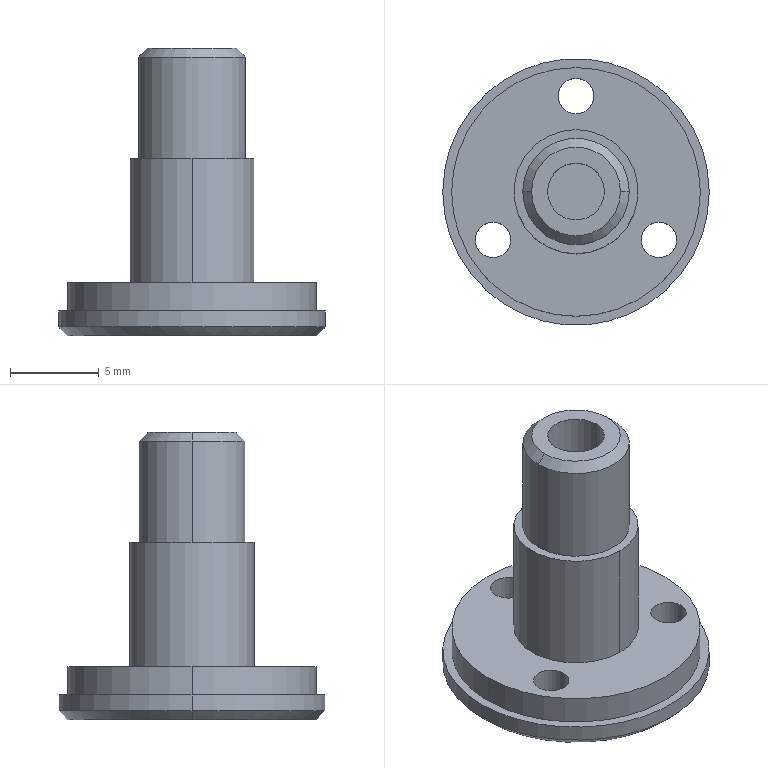Part | NX | features BREP 1 | 1 solid | 26 faces | box 15 x 15 x 16.2 mm | volume 821.71 mm3 | cylinder 16 | plane 6 | cone 4 | commonest cylinder face diameters 2 x6 3.2 x2 6 x2 7 x2 14 x2 15 x2
STEP:
#1=CARTESIAN_POINT('',(54.808,248.839,0.));
#2=VERTEX_POINT('',#1);
#3=CARTESIAN_POINT('',(49.808,248.839,0.));
#4=VERTEX_POINT('',#3);
#5=CARTESIAN_POINT('',(52.308,248.839,0.));
#6=DIRECTION('',(0.,0.,1.));
#7=DIRECTION('',(1.,0.,0.));
#8=AXIS2_PLACEMENT_3D('',#5,#6,#7);
#9=CIRCLE('',#8,2.5);
#10=EDGE_CURVE('',#2,#4,#9,.T.);
#11=ORIENTED_EDGE('',*,*,#10,.F.);
#12=CARTESIAN_POINT('',(55.308,248.839,-0.5));
#13=VERTEX_POINT('',#12);
#14=CARTESIAN_POINT('',(54.808,248.839,0.));
#15=DIRECTION('',(0.7071,0.,-0.7071));
#16=VECTOR('',#15,1000.);
#17=LINE('',#14,#16);
#18=EDGE_CURVE('',#13,#2,#17,.F.);
#19=ORIENTED_EDGE('',*,*,#18,.F.);
#20=CARTESIAN_POINT('',(49.308,248.839,-0.5));
#21=VERTEX_POINT('',#20);
#22=CARTESIAN_POINT('',(52.308,248.839,-0.5));
#23=DIRECTION('',(0.,0.,-1.));
#24=DIRECTION('',(1.,0.,0.));
#25=AXIS2_PLACEMENT_3D('',#22,#23,#24);
#26=CIRCLE('',#25,3.);
#27=EDGE_CURVE('',#21,#13,#26,.T.);
#28=ORIENTED_EDGE('',*,*,#27,.F.);
#29=CARTESIAN_POINT('',(49.808,248.839,0.));
#30=DIRECTION('',(-0.7071,0.,-0.7071));
#31=VECTOR('',#30,1000.);
#32=LINE('',#29,#31);
#33=EDGE_CURVE('',#21,#4,#32,.F.);
#34=ORIENTED_EDGE('',*,*,#33,.T.);
#35=EDGE_LOOP('',(#11,#19,#28,#34));
#36=FACE_BOUND('',#35,.T.);
#37=CARTESIAN_POINT('',(52.308,248.839,0.));
#38=DIRECTION('',(0.,0.,-1.));
#39=DIRECTION('',(1.,0.,0.));
#40=AXIS2_PLACEMENT_3D('',#37,#38,#39);
#41=CONICAL_SURFACE('',#40,2.5,0.7854);
#42=ADVANCED_FACE('',(#36),#41,.T.);
#43=CARTESIAN_POINT('',(50.708,248.839,-10.));
#44=VERTEX_POINT('',#43);
#45=CARTESIAN_POINT('',(53.908,248.839,-10.));
#46=VERTEX_POINT('',#45);
#47=CARTESIAN_POINT('',(52.308,248.839,-10.));
#48=DIRECTION('',(0.,0.,1.));
#49=DIRECTION('',(1.,0.,0.));
#50=AXIS2_PLACEMENT_3D('',#47,#48,#49);
#51=CIRCLE('',#50,1.6);
#52=EDGE_CURVE('',#44,#46,#51,.T.);
#53=ORIENTED_EDGE('',*,*,#52,.F.);
#54=CARTESIAN_POINT('',(50.708,248.839,0.));
#55=VERTEX_POINT('',#54);
#56=CARTESIAN_POINT('',(50.708,248.839,-10.));
#57=DIRECTION('',(0.,0.,1.));
#58=VECTOR('',#57,1000.);
#59=LINE('',#56,#58);
#60=EDGE_CURVE('',#44,#55,#59,.T.);
#61=ORIENTED_EDGE('',*,*,#60,.T.);
#62=CARTESIAN_POINT('',(53.908,248.839,0.));
#63=VERTEX_POINT('',#62);
#64=CARTESIAN_POINT('',(52.308,248.839,0.));
#65=DIRECTION('',(0.,0.,1.));
#66=DIRECTION('',(1.,0.,0.));
#67=AXIS2_PLACEMENT_3D('',#64,#65,#66);
#68=CIRCLE('',#67,1.6);
#69=EDGE_CURVE('',#55,#63,#68,.T.);
#70=ORIENTED_EDGE('',*,*,#69,.T.);
#71=CARTESIAN_POINT('',(53.908,248.839,-10.));
#72=DIRECTION('',(0.,0.,1.));
#73=VECTOR('',#72,1000.);
#74=LINE('',#71,#73);
#75=EDGE_CURVE('',#46,#63,#74,.T.);
#76=ORIENTED_EDGE('',*,*,#75,.F.);
#77=EDGE_LOOP('',(#53,#61,#70,#76));
#78=FACE_BOUND('',#77,.T.);
#79=CARTESIAN_POINT('',(52.308,248.839,-10.));
#80=DIRECTION('',(0.,0.,1.));
#81=DIRECTION('',(-1.,0.,0.));
#82=AXIS2_PLACEMENT_3D('',#79,#80,#81);
#83=CYLINDRICAL_SURFACE('',#82,1.6);
#84=ADVANCED_FACE('',(#78),#83,.F.);
#85=CARTESIAN_POINT('',(45.308,248.839,-16.2));
#86=VERTEX_POINT('',#85);
#87=CARTESIAN_POINT('',(59.308,248.839,-16.2));
#88=VERTEX_POINT('',#87);
#89=CARTESIAN_POINT('',(52.308,248.839,-16.2));
#90=DIRECTION('',(0.,0.,-1.));
#91=DIRECTION('',(0.,1.,0.));
#92=AXIS2_PLACEMENT_3D('',#89,#90,#91);
#93=CIRCLE('',#92,7.);
#94=EDGE_CURVE('',#86,#88,#93,.T.);
#95=ORIENTED_EDGE('',*,*,#94,.F.);
#96=CARTESIAN_POINT('',(44.808,248.839,-15.7));
#97=VERTEX_POINT('',#96);
#98=CARTESIAN_POINT('',(45.308,248.839,-16.2));
#99=DIRECTION('',(-0.7071,0.,0.7071));
#100=VECTOR('',#99,1000.);
#101=LINE('',#98,#100);
#102=EDGE_CURVE('',#86,#97,#101,.T.);
#103=ORIENTED_EDGE('',*,*,#102,.T.);
#104=CARTESIAN_POINT('',(59.808,248.839,-15.7));
#105=VERTEX_POINT('',#104);
#106=CARTESIAN_POINT('',(52.308,248.839,-15.7));
#107=DIRECTION('',(0.,0.,1.));
#108=DIRECTION('',(-1.,0.,0.));
#109=AXIS2_PLACEMENT_3D('',#106,#107,#108);
#110=CIRCLE('',#109,7.5);
#111=EDGE_CURVE('',#105,#97,#110,.T.);
#112=ORIENTED_EDGE('',*,*,#111,.F.);
#113=CARTESIAN_POINT('',(59.308,248.839,-16.2));
#114=DIRECTION('',(0.7071,0.,0.7071));
#115=VECTOR('',#114,1000.);
#116=LINE('',#113,#115);
#117=EDGE_CURVE('',#88,#105,#116,.T.);
#118=ORIENTED_EDGE('',*,*,#117,.F.);
#119=EDGE_LOOP('',(#95,#103,#112,#118));
#120=FACE_BOUND('',#119,.T.);
#121=CARTESIAN_POINT('',(52.308,248.839,-16.2));
#122=DIRECTION('',(0.,0.,1.));
#123=DIRECTION('',(-1.,0.,0.));
#124=AXIS2_PLACEMENT_3D('',#121,#122,#123);
#125=CONICAL_SURFACE('',#124,7.,0.7854);
#126=ADVANCED_FACE('',(#120),#125,.T.);
#127=ORIENTED_EDGE('',*,*,#111,.T.);
#128=CARTESIAN_POINT('',(44.808,248.839,-14.8));
#129=VERTEX_POINT('',#128);
#130=CARTESIAN_POINT('',(44.808,248.839,-36.413));
#131=DIRECTION('',(0.,0.,1.));
#132=VECTOR('',#131,1000.);
#133=LINE('',#130,#132);
#134=EDGE_CURVE('',#97,#129,#133,.T.);
#135=ORIENTED_EDGE('',*,*,#134,.T.);
#136=CARTESIAN_POINT('',(59.808,248.839,-14.8));
#137=VERTEX_POINT('',#136);
#138=CARTESIAN_POINT('',(52.308,248.839,-14.8));
#139=DIRECTION('',(0.,0.,-1.));
#140=DIRECTION('',(-1.,0.,0.));
#141=AXIS2_PLACEMENT_3D('',#138,#139,#140);
#142=CIRCLE('',#141,7.5);
#143=EDGE_CURVE('',#129,#137,#142,.T.);
#144=ORIENTED_EDGE('',*,*,#143,.T.);
#145=CARTESIAN_POINT('',(59.808,248.839,-36.413));
#146=DIRECTION('',(0.,0.,1.));
#147=VECTOR('',#146,1000.);
#148=LINE('',#145,#147);
#149=EDGE_CURVE('',#105,#137,#148,.T.);
#150=ORIENTED_EDGE('',*,*,#149,.F.);
#151=EDGE_LOOP('',(#127,#135,#144,#150));
#152=FACE_BOUND('',#151,.T.);
#153=CARTESIAN_POINT('',(52.308,248.839,-36.413));
#154=DIRECTION('',(0.,0.,1.));
#155=DIRECTION('',(-1.,0.,0.));
#156=AXIS2_PLACEMENT_3D('',#153,#154,#155);
#157=CYLINDRICAL_SURFACE('',#156,7.5);
#158=ADVANCED_FACE('',(#152),#157,.T.);
#159=CARTESIAN_POINT('',(53.308,254.236,-13.2));
#160=VERTEX_POINT('',#159);
#161=CARTESIAN_POINT('',(51.308,254.236,-13.2));
#162=VERTEX_POINT('',#161);
#163=CARTESIAN_POINT('',(52.308,254.236,-13.2));
#164=DIRECTION('',(0.,0.,-1.));
#165=DIRECTION('',(-1.,0.,0.));
#166=AXIS2_PLACEMENT_3D('',#163,#164,#165);
#167=CIRCLE('',#166,1.);
#168=EDGE_CURVE('',#160,#162,#167,.T.);
#169=ORIENTED_EDGE('',*,*,#168,.F.);
#170=CARTESIAN_POINT('',(53.308,254.236,-16.2));
#171=VERTEX_POINT('',#170);
#172=CARTESIAN_POINT('',(53.308,254.236,-4.3));
#173=DIRECTION('',(0.,0.,-1.));
#174=VECTOR('',#173,1000.);
#175=LINE('',#172,#174);
#176=EDGE_CURVE('',#171,#160,#175,.F.);
#177=ORIENTED_EDGE('',*,*,#176,.F.);
#178=CARTESIAN_POINT('',(51.308,254.236,-16.2));
#179=VERTEX_POINT('',#178);
#180=CARTESIAN_POINT('',(52.308,254.236,-16.2));
#181=DIRECTION('',(0.,0.,-1.));
#182=DIRECTION('',(0.,1.,0.));
#183=AXIS2_PLACEMENT_3D('',#180,#181,#182);
#184=CIRCLE('',#183,1.);
#185=EDGE_CURVE('',#171,#179,#184,.T.);
#186=ORIENTED_EDGE('',*,*,#185,.T.);
#187=CARTESIAN_POINT('',(51.308,254.236,-4.3));
#188=DIRECTION('',(0.,0.,-1.));
#189=VECTOR('',#188,1000.);
#190=LINE('',#187,#189);
#191=EDGE_CURVE('',#179,#162,#190,.F.);
#192=ORIENTED_EDGE('',*,*,#191,.T.);
#193=EDGE_LOOP('',(#169,#177,#186,#192));
#194=FACE_BOUND('',#193,.T.);
#195=CARTESIAN_POINT('',(52.308,254.236,-4.3));
#196=DIRECTION('',(0.,0.,-1.));
#197=DIRECTION('',(1.,0.,0.));
#198=AXIS2_PLACEMENT_3D('',#195,#196,#197);
#199=CYLINDRICAL_SURFACE('',#198,1.);
#200=ADVANCED_FACE('',(#194),#199,.F.);
#201=CARTESIAN_POINT('',(48.633,246.14,-13.2));
#202=VERTEX_POINT('',#201);
#203=CARTESIAN_POINT('',(46.633,246.14,-13.2));
#204=VERTEX_POINT('',#203);
#205=CARTESIAN_POINT('',(47.633,246.14,-13.2));
#206=DIRECTION('',(0.,0.,-1.));
#207=DIRECTION('',(-1.,0.,0.));
#208=AXIS2_PLACEMENT_3D('',#205,#206,#207);
#209=CIRCLE('',#208,1.);
#210=EDGE_CURVE('',#202,#204,#209,.T.);
#211=ORIENTED_EDGE('',*,*,#210,.F.);
#212=CARTESIAN_POINT('',(48.633,246.14,-16.2));
#213=VERTEX_POINT('',#212);
#214=CARTESIAN_POINT('',(48.633,246.14,-4.3));
#215=DIRECTION('',(0.,0.,-1.));
#216=VECTOR('',#215,1000.);
#217=LINE('',#214,#216);
#218=EDGE_CURVE('',#213,#202,#217,.F.);
#219=ORIENTED_EDGE('',*,*,#218,.F.);
#220=CARTESIAN_POINT('',(46.633,246.14,-16.2));
#221=VERTEX_POINT('',#220);
#222=CARTESIAN_POINT('',(47.633,246.14,-16.2));
#223=DIRECTION('',(0.,0.,-1.));
#224=DIRECTION('',(0.,1.,0.));
#225=AXIS2_PLACEMENT_3D('',#222,#223,#224);
#226=CIRCLE('',#225,1.);
#227=EDGE_CURVE('',#213,#221,#226,.T.);
#228=ORIENTED_EDGE('',*,*,#227,.T.);
#229=CARTESIAN_POINT('',(46.633,246.14,-4.3));
#230=DIRECTION('',(0.,0.,-1.));
#231=VECTOR('',#230,1000.);
#232=LINE('',#229,#231);
#233=EDGE_CURVE('',#221,#204,#232,.F.);
#234=ORIENTED_EDGE('',*,*,#233,.T.);
#235=EDGE_LOOP('',(#211,#219,#228,#234));
#236=FACE_BOUND('',#235,.T.);
#237=CARTESIAN_POINT('',(47.633,246.14,-4.3));
#238=DIRECTION('',(0.,0.,-1.));
#239=DIRECTION('',(1.,0.,0.));
#240=AXIS2_PLACEMENT_3D('',#237,#238,#239);
#241=CYLINDRICAL_SURFACE('',#240,1.);
#242=ADVANCED_FACE('',(#236),#241,.F.);
#243=CARTESIAN_POINT('',(57.982,246.14,-13.2));
#244=VERTEX_POINT('',#243);
#245=CARTESIAN_POINT('',(55.982,246.14,-13.2));
#246=VERTEX_POINT('',#245);
#247=CARTESIAN_POINT('',(56.982,246.14,-13.2));
#248=DIRECTION('',(0.,0.,-1.));
#249=DIRECTION('',(-1.,0.,0.));
#250=AXIS2_PLACEMENT_3D('',#247,#248,#249);
#251=CIRCLE('',#250,1.);
#252=EDGE_CURVE('',#244,#246,#251,.T.);
#253=ORIENTED_EDGE('',*,*,#252,.F.);
#254=CARTESIAN_POINT('',(57.982,246.14,-16.2));
#255=VERTEX_POINT('',#254);
#256=CARTESIAN_POINT('',(57.982,246.14,-4.3));
#257=DIRECTION('',(0.,0.,-1.));
#258=VECTOR('',#257,1000.);
#259=LINE('',#256,#258);
#260=EDGE_CURVE('',#255,#244,#259,.F.);
#261=ORIENTED_EDGE('',*,*,#260,.F.);
#262=CARTESIAN_POINT('',(55.982,246.14,-16.2));
#263=VERTEX_POINT('',#262);
#264=CARTESIAN_POINT('',(56.982,246.14,-16.2));
#265=DIRECTION('',(0.,0.,-1.));
#266=DIRECTION('',(0.,1.,0.));
#267=AXIS2_PLACEMENT_3D('',#264,#265,#266);
#268=CIRCLE('',#267,1.);
#269=EDGE_CURVE('',#255,#263,#268,.T.);
#270=ORIENTED_EDGE('',*,*,#269,.T.);
#271=CARTESIAN_POINT('',(55.982,246.14,-4.3));
#272=DIRECTION('',(0.,0.,-1.));
#273=VECTOR('',#272,1000.);
#274=LINE('',#271,#273);
#275=EDGE_CURVE('',#263,#246,#274,.F.);
#276=ORIENTED_EDGE('',*,*,#275,.T.);
#277=EDGE_LOOP('',(#253,#261,#270,#276));
#278=FACE_BOUND('',#277,.T.);
#279=CARTESIAN_POINT('',(56.982,246.14,-4.3));
#280=DIRECTION('',(0.,0.,-1.));
#281=DIRECTION('',(1.,0.,0.));
#282=AXIS2_PLACEMENT_3D('',#279,#280,#281);
#283=CYLINDRICAL_SURFACE('',#282,1.);
#284=ADVANCED_FACE('',(#278),#283,.F.);
#285=CARTESIAN_POINT('',(45.308,248.839,-14.8));
#286=VERTEX_POINT('',#285);
#287=CARTESIAN_POINT('',(59.308,248.839,-14.8));
#288=VERTEX_POINT('',#287);
#289=CARTESIAN_POINT('',(52.308,248.839,-14.8));
#290=DIRECTION('',(0.,0.,-1.));
#291=DIRECTION('',(-1.,0.,0.));
#292=AXIS2_PLACEMENT_3D('',#289,#290,#291);
#293=CIRCLE('',#292,7.);
#294=EDGE_CURVE('',#286,#288,#293,.T.);
#295=ORIENTED_EDGE('',*,*,#294,.F.);
#296=CARTESIAN_POINT('',(45.308,248.839,-13.2));
#297=VERTEX_POINT('',#296);
#298=CARTESIAN_POINT('',(45.308,248.839,-34.099));
#299=DIRECTION('',(0.,0.,1.));
#300=VECTOR('',#299,1000.);
#301=LINE('',#298,#300);
#302=EDGE_CURVE('',#286,#297,#301,.T.);
#303=ORIENTED_EDGE('',*,*,#302,.T.);
#304=CARTESIAN_POINT('',(59.308,248.839,-13.2));
#305=VERTEX_POINT('',#304);
#306=CARTESIAN_POINT('',(52.308,248.839,-13.2));
#307=DIRECTION('',(0.,0.,-1.));
#308=DIRECTION('',(-1.,0.,0.));
#309=AXIS2_PLACEMENT_3D('',#306,#307,#308);
#310=CIRCLE('',#309,7.);
#311=EDGE_CURVE('',#297,#305,#310,.T.);
#312=ORIENTED_EDGE('',*,*,#311,.T.);
#313=CARTESIAN_POINT('',(59.308,248.839,-34.099));
#314=DIRECTION('',(0.,0.,1.));
#315=VECTOR('',#314,1000.);
#316=LINE('',#313,#315);
#317=EDGE_CURVE('',#288,#305,#316,.T.);
#318=ORIENTED_EDGE('',*,*,#317,.F.);
#319=EDGE_LOOP('',(#295,#303,#312,#318));
#320=FACE_BOUND('',#319,.T.);
#321=CARTESIAN_POINT('',(52.308,248.839,-34.099));
#322=DIRECTION('',(0.,0.,1.));
#323=DIRECTION('',(-1.,0.,0.));
#324=AXIS2_PLACEMENT_3D('',#321,#322,#323);
#325=CYLINDRICAL_SURFACE('',#324,7.);
#326=ADVANCED_FACE('',(#320),#325,.T.);
#327=CARTESIAN_POINT('',(52.308,245.339,-13.2));
#328=VERTEX_POINT('',#327);
#329=CARTESIAN_POINT('',(52.308,252.339,-13.2));
#330=VERTEX_POINT('',#329);
#331=CARTESIAN_POINT('',(52.308,248.839,-13.2));
#332=DIRECTION('',(0.,0.,1.));
#333=DIRECTION('',(-1.,0.,0.));
#334=AXIS2_PLACEMENT_3D('',#331,#332,#333);
#335=CIRCLE('',#334,3.5);
#336=EDGE_CURVE('',#328,#330,#335,.T.);
#337=ORIENTED_EDGE('',*,*,#336,.T.);
#338=CARTESIAN_POINT('',(52.308,252.339,-6.2));
#339=VERTEX_POINT('',#338);
#340=CARTESIAN_POINT('',(52.308,252.339,-24.014));
#341=DIRECTION('',(0.,0.,1.));
#342=VECTOR('',#341,1000.);
#343=LINE('',#340,#342);
#344=EDGE_CURVE('',#339,#330,#343,.F.);
#345=ORIENTED_EDGE('',*,*,#344,.F.);
#346=CARTESIAN_POINT('',(52.308,245.339,-6.2));
#347=VERTEX_POINT('',#346);
#348=CARTESIAN_POINT('',(52.308,248.839,-6.2));
#349=DIRECTION('',(0.,0.,-1.));
#350=DIRECTION('',(0.,1.,0.));
#351=AXIS2_PLACEMENT_3D('',#348,#349,#350);
#352=CIRCLE('',#351,3.5);
#353=EDGE_CURVE('',#339,#347,#352,.T.);
#354=ORIENTED_EDGE('',*,*,#353,.T.);
#355=CARTESIAN_POINT('',(52.308,245.339,-24.014));
#356=DIRECTION('',(0.,0.,1.));
#357=VECTOR('',#356,1000.);
#358=LINE('',#355,#357);
#359=EDGE_CURVE('',#347,#328,#358,.F.);
#360=ORIENTED_EDGE('',*,*,#359,.T.);
#361=EDGE_LOOP('',(#337,#345,#354,#360));
#362=FACE_BOUND('',#361,.T.);
#363=CARTESIAN_POINT('',(52.308,248.839,-24.014));
#364=DIRECTION('',(0.,0.,1.));
#365=DIRECTION('',(0.,1.,0.));
#366=AXIS2_PLACEMENT_3D('',#363,#364,#365);
#367=CYLINDRICAL_SURFACE('',#366,3.5);
#368=ADVANCED_FACE('',(#362),#367,.T.);
#369=CARTESIAN_POINT('',(49.308,248.839,-6.2));
#370=VERTEX_POINT('',#369);
#371=CARTESIAN_POINT('',(55.308,248.839,-6.2));
#372=VERTEX_POINT('',#371);
#373=CARTESIAN_POINT('',(52.308,248.839,-6.2));
#374=DIRECTION('',(0.,0.,-1.));
#375=DIRECTION('',(0.,1.,0.));
#376=AXIS2_PLACEMENT_3D('',#373,#374,#375);
#377=CIRCLE('',#376,3.);
#378=EDGE_CURVE('',#370,#372,#377,.T.);
#379=ORIENTED_EDGE('',*,*,#378,.F.);
#380=CARTESIAN_POINT('',(49.308,248.839,-15.085));
#381=DIRECTION('',(0.,0.,1.));
#382=VECTOR('',#381,1000.);
#383=LINE('',#380,#382);
#384=EDGE_CURVE('',#370,#21,#383,.T.);
#385=ORIENTED_EDGE('',*,*,#384,.T.);
#386=ORIENTED_EDGE('',*,*,#27,.T.);
#387=CARTESIAN_POINT('',(55.308,248.839,-15.085));
#388=DIRECTION('',(0.,0.,1.));
#389=VECTOR('',#388,1000.);
#390=LINE('',#387,#389);
#391=EDGE_CURVE('',#372,#13,#390,.T.);
#392=ORIENTED_EDGE('',*,*,#391,.F.);
#393=EDGE_LOOP('',(#379,#385,#386,#392));
#394=FACE_BOUND('',#393,.T.);
#395=CARTESIAN_POINT('',(52.308,248.839,-15.085));
#396=DIRECTION('',(0.,0.,1.));
#397=DIRECTION('',(-1.,0.,0.));
#398=AXIS2_PLACEMENT_3D('',#395,#396,#397);
#399=CYLINDRICAL_SURFACE('',#398,3.);
#400=ADVANCED_FACE('',(#394),#399,.T.);
#401=ORIENTED_EDGE('',*,*,#384,.F.);
#402=CARTESIAN_POINT('',(52.308,248.839,-6.2));
#403=DIRECTION('',(0.,0.,-1.));
#404=DIRECTION('',(0.,1.,0.));
#405=AXIS2_PLACEMENT_3D('',#402,#403,#404);
#406=CIRCLE('',#405,3.);
#407=EDGE_CURVE('',#372,#370,#406,.T.);
#408=ORIENTED_EDGE('',*,*,#407,.F.);
#409=ORIENTED_EDGE('',*,*,#391,.T.);
#410=CARTESIAN_POINT('',(52.308,248.839,-0.5));
#411=DIRECTION('',(0.,0.,-1.));
#412=DIRECTION('',(1.,0.,0.));
#413=AXIS2_PLACEMENT_3D('',#410,#411,#412);
#414=CIRCLE('',#413,3.);
#415=EDGE_CURVE('',#13,#21,#414,.T.);
#416=ORIENTED_EDGE('',*,*,#415,.T.);
#417=EDGE_LOOP('',(#401,#408,#409,#416));
#418=FACE_BOUND('',#417,.T.);
#419=CARTESIAN_POINT('',(52.308,248.839,-15.085));
#420=DIRECTION('',(0.,0.,1.));
#421=DIRECTION('',(-1.,0.,0.));
#422=AXIS2_PLACEMENT_3D('',#419,#420,#421);
#423=CYLINDRICAL_SURFACE('',#422,3.);
#424=ADVANCED_FACE('',(#418),#423,.T.);
#425=CARTESIAN_POINT('',(52.308,248.839,0.));
#426=DIRECTION('',(0.,0.,1.));
#427=DIRECTION('',(1.,0.,0.));
#428=AXIS2_PLACEMENT_3D('',#425,#426,#427);
#429=CIRCLE('',#428,2.5);
#430=EDGE_CURVE('',#4,#2,#429,.T.);
#431=ORIENTED_EDGE('',*,*,#430,.T.);
#432=ORIENTED_EDGE('',*,*,#10,.T.);
#433=EDGE_LOOP('',(#431,#432));
#434=FACE_BOUND('',#433,.T.);
#435=CARTESIAN_POINT('',(52.308,248.839,0.));
#436=DIRECTION('',(0.,0.,1.));
#437=DIRECTION('',(1.,0.,0.));
#438=AXIS2_PLACEMENT_3D('',#435,#436,#437);
#439=CIRCLE('',#438,1.6);
#440=EDGE_CURVE('',#63,#55,#439,.T.);
#441=ORIENTED_EDGE('',*,*,#440,.F.);
#442=ORIENTED_EDGE('',*,*,#69,.F.);
#443=EDGE_LOOP('',(#441,#442));
#444=FACE_BOUND('',#443,.T.);
#445=CARTESIAN_POINT('',(52.308,248.839,0.));
#446=DIRECTION('',(0.,0.,1.));
#447=DIRECTION('',(-1.,0.,0.));
#448=AXIS2_PLACEMENT_3D('',#445,#446,#447);
#449=PLANE('',#448);
#450=ADVANCED_FACE('',(#434,#444),#449,.T.);
#451=CARTESIAN_POINT('',(52.308,248.839,-6.2));
#452=DIRECTION('',(0.,0.,-1.));
#453=DIRECTION('',(0.,1.,0.));
#454=AXIS2_PLACEMENT_3D('',#451,#452,#453);
#455=CIRCLE('',#454,3.5);
#456=EDGE_CURVE('',#347,#339,#455,.T.);
#457=ORIENTED_EDGE('',*,*,#456,.F.);
#458=ORIENTED_EDGE('',*,*,#353,.F.);
#459=EDGE_LOOP('',(#457,#458));
#460=FACE_BOUND('',#459,.T.);
#461=ORIENTED_EDGE('',*,*,#407,.T.);
#462=ORIENTED_EDGE('',*,*,#378,.T.);
#463=EDGE_LOOP('',(#461,#462));
#464=FACE_BOUND('',#463,.T.);
#465=CARTESIAN_POINT('',(52.308,248.839,-6.2));
#466=DIRECTION('',(0.,0.,-1.));
#467=DIRECTION('',(0.,1.,0.));
#468=AXIS2_PLACEMENT_3D('',#465,#466,#467);
#469=PLANE('',#468);
#470=ADVANCED_FACE('',(#460,#464),#469,.F.);
#471=ORIENTED_EDGE('',*,*,#344,.T.);
#472=CARTESIAN_POINT('',(52.308,248.839,-13.2));
#473=DIRECTION('',(0.,0.,1.));
#474=DIRECTION('',(-1.,0.,0.));
#475=AXIS2_PLACEMENT_3D('',#472,#473,#474);
#476=CIRCLE('',#475,3.5);
#477=EDGE_CURVE('',#330,#328,#476,.T.);
#478=ORIENTED_EDGE('',*,*,#477,.T.);
#479=ORIENTED_EDGE('',*,*,#359,.F.);
#480=ORIENTED_EDGE('',*,*,#456,.T.);
#481=EDGE_LOOP('',(#471,#478,#479,#480));
#482=FACE_BOUND('',#481,.T.);
#483=CARTESIAN_POINT('',(52.308,248.839,-24.014));
#484=DIRECTION('',(0.,0.,1.));
#485=DIRECTION('',(0.,1.,0.));
#486=AXIS2_PLACEMENT_3D('',#483,#484,#485);
#487=CYLINDRICAL_SURFACE('',#486,3.5);
#488=ADVANCED_FACE('',(#482),#487,.T.);
#489=ORIENTED_EDGE('',*,*,#302,.F.);
#490=CARTESIAN_POINT('',(52.308,248.839,-14.8));
#491=DIRECTION('',(0.,0.,-1.));
#492=DIRECTION('',(-1.,0.,0.));
#493=AXIS2_PLACEMENT_3D('',#490,#491,#492);
#494=CIRCLE('',#493,7.);
#495=EDGE_CURVE('',#288,#286,#494,.T.);
#496=ORIENTED_EDGE('',*,*,#495,.F.);
#497=ORIENTED_EDGE('',*,*,#317,.T.);
#498=CARTESIAN_POINT('',(52.308,248.839,-13.2));
#499=DIRECTION('',(0.,0.,-1.));
#500=DIRECTION('',(-1.,0.,0.));
#501=AXIS2_PLACEMENT_3D('',#498,#499,#500);
#502=CIRCLE('',#501,7.);
#503=EDGE_CURVE('',#305,#297,#502,.T.);
#504=ORIENTED_EDGE('',*,*,#503,.T.);
#505=EDGE_LOOP('',(#489,#496,#497,#504));
#506=FACE_BOUND('',#505,.T.);
#507=CARTESIAN_POINT('',(52.308,248.839,-34.099));
#508=DIRECTION('',(0.,0.,1.));
#509=DIRECTION('',(-1.,0.,0.));
#510=AXIS2_PLACEMENT_3D('',#507,#508,#509);
#511=CYLINDRICAL_SURFACE('',#510,7.);
#512=ADVANCED_FACE('',(#506),#511,.T.);
#513=ORIENTED_EDGE('',*,*,#503,.F.);
#514=ORIENTED_EDGE('',*,*,#311,.F.);
#515=EDGE_LOOP('',(#513,#514));
#516=FACE_BOUND('',#515,.T.);
#517=CARTESIAN_POINT('',(52.308,254.236,-13.2));
#518=DIRECTION('',(0.,0.,-1.));
#519=DIRECTION('',(-1.,0.,0.));
#520=AXIS2_PLACEMENT_3D('',#517,#518,#519);
#521=CIRCLE('',#520,1.);
#522=EDGE_CURVE('',#162,#160,#521,.T.);
#523=ORIENTED_EDGE('',*,*,#522,.T.);
#524=ORIENTED_EDGE('',*,*,#168,.T.);
#525=EDGE_LOOP('',(#523,#524));
#526=FACE_BOUND('',#525,.T.);
#527=CARTESIAN_POINT('',(47.633,246.14,-13.2));
#528=DIRECTION('',(0.,0.,-1.));
#529=DIRECTION('',(-1.,0.,0.));
#530=AXIS2_PLACEMENT_3D('',#527,#528,#529);
#531=CIRCLE('',#530,1.);
#532=EDGE_CURVE('',#204,#202,#531,.T.);
#533=ORIENTED_EDGE('',*,*,#532,.T.);
#534=ORIENTED_EDGE('',*,*,#210,.T.);
#535=EDGE_LOOP('',(#533,#534));
#536=FACE_BOUND('',#535,.T.);
#537=CARTESIAN_POINT('',(56.982,246.14,-13.2));
#538=DIRECTION('',(0.,0.,-1.));
#539=DIRECTION('',(-1.,0.,0.));
#540=AXIS2_PLACEMENT_3D('',#537,#538,#539);
#541=CIRCLE('',#540,1.);
#542=EDGE_CURVE('',#246,#244,#541,.T.);
#543=ORIENTED_EDGE('',*,*,#542,.T.);
#544=ORIENTED_EDGE('',*,*,#252,.T.);
#545=EDGE_LOOP('',(#543,#544));
#546=FACE_BOUND('',#545,.T.);
#547=ORIENTED_EDGE('',*,*,#336,.F.);
#548=ORIENTED_EDGE('',*,*,#477,.F.);
#549=EDGE_LOOP('',(#547,#548));
#550=FACE_BOUND('',#549,.T.);
#551=CARTESIAN_POINT('',(52.308,248.839,-13.2));
#552=DIRECTION('',(0.,0.,-1.));
#553=DIRECTION('',(1.,0.,0.));
#554=AXIS2_PLACEMENT_3D('',#551,#552,#553);
#555=PLANE('',#554);
#556=ADVANCED_FACE('',(#516,#526,#536,#546,#550),#555,.F.);
#557=ORIENTED_EDGE('',*,*,#260,.T.);
#558=ORIENTED_EDGE('',*,*,#542,.F.);
#559=ORIENTED_EDGE('',*,*,#275,.F.);
#560=CARTESIAN_POINT('',(56.982,246.14,-16.2));
#561=DIRECTION('',(0.,0.,-1.));
#562=DIRECTION('',(0.,1.,0.));
#563=AXIS2_PLACEMENT_3D('',#560,#561,#562);
#564=CIRCLE('',#563,1.);
#565=EDGE_CURVE('',#263,#255,#564,.T.);
#566=ORIENTED_EDGE('',*,*,#565,.T.);
#567=EDGE_LOOP('',(#557,#558,#559,#566));
#568=FACE_BOUND('',#567,.T.);
#569=CARTESIAN_POINT('',(56.982,246.14,-4.3));
#570=DIRECTION('',(0.,0.,-1.));
#571=DIRECTION('',(1.,0.,0.));
#572=AXIS2_PLACEMENT_3D('',#569,#570,#571);
#573=CYLINDRICAL_SURFACE('',#572,1.);
#574=ADVANCED_FACE('',(#568),#573,.F.);
#575=ORIENTED_EDGE('',*,*,#218,.T.);
#576=ORIENTED_EDGE('',*,*,#532,.F.);
#577=ORIENTED_EDGE('',*,*,#233,.F.);
#578=CARTESIAN_POINT('',(47.633,246.14,-16.2));
#579=DIRECTION('',(0.,0.,-1.));
#580=DIRECTION('',(0.,1.,0.));
#581=AXIS2_PLACEMENT_3D('',#578,#579,#580);
#582=CIRCLE('',#581,1.);
#583=EDGE_CURVE('',#221,#213,#582,.T.);
#584=ORIENTED_EDGE('',*,*,#583,.T.);
#585=EDGE_LOOP('',(#575,#576,#577,#584));
#586=FACE_BOUND('',#585,.T.);
#587=CARTESIAN_POINT('',(47.633,246.14,-4.3));
#588=DIRECTION('',(0.,0.,-1.));
#589=DIRECTION('',(1.,0.,0.));
#590=AXIS2_PLACEMENT_3D('',#587,#588,#589);
#591=CYLINDRICAL_SURFACE('',#590,1.);
#592=ADVANCED_FACE('',(#586),#591,.F.);
#593=ORIENTED_EDGE('',*,*,#176,.T.);
#594=ORIENTED_EDGE('',*,*,#522,.F.);
#595=ORIENTED_EDGE('',*,*,#191,.F.);
#596=CARTESIAN_POINT('',(52.308,254.236,-16.2));
#597=DIRECTION('',(0.,0.,-1.));
#598=DIRECTION('',(0.,1.,0.));
#599=AXIS2_PLACEMENT_3D('',#596,#597,#598);
#600=CIRCLE('',#599,1.);
#601=EDGE_CURVE('',#179,#171,#600,.T.);
#602=ORIENTED_EDGE('',*,*,#601,.T.);
#603=EDGE_LOOP('',(#593,#594,#595,#602));
#604=FACE_BOUND('',#603,.T.);
#605=CARTESIAN_POINT('',(52.308,254.236,-4.3));
#606=DIRECTION('',(0.,0.,-1.));
#607=DIRECTION('',(1.,0.,0.));
#608=AXIS2_PLACEMENT_3D('',#605,#606,#607);
#609=CYLINDRICAL_SURFACE('',#608,1.);
#610=ADVANCED_FACE('',(#604),#609,.F.);
#611=ORIENTED_EDGE('',*,*,#134,.F.);
#612=CARTESIAN_POINT('',(52.308,248.839,-15.7));
#613=DIRECTION('',(0.,0.,1.));
#614=DIRECTION('',(-1.,0.,0.));
#615=AXIS2_PLACEMENT_3D('',#612,#613,#614);
#616=CIRCLE('',#615,7.5);
#617=EDGE_CURVE('',#97,#105,#616,.T.);
#618=ORIENTED_EDGE('',*,*,#617,.T.);
#619=ORIENTED_EDGE('',*,*,#149,.T.);
#620=CARTESIAN_POINT('',(52.308,248.839,-14.8));
#621=DIRECTION('',(0.,0.,-1.));
#622=DIRECTION('',(-1.,0.,0.));
#623=AXIS2_PLACEMENT_3D('',#620,#621,#622);
#624=CIRCLE('',#623,7.5);
#625=EDGE_CURVE('',#137,#129,#624,.T.);
#626=ORIENTED_EDGE('',*,*,#625,.T.);
#627=EDGE_LOOP('',(#611,#618,#619,#626));
#628=FACE_BOUND('',#627,.T.);
#629=CARTESIAN_POINT('',(52.308,248.839,-36.413));
#630=DIRECTION('',(0.,0.,1.));
#631=DIRECTION('',(-1.,0.,0.));
#632=AXIS2_PLACEMENT_3D('',#629,#630,#631);
#633=CYLINDRICAL_SURFACE('',#632,7.5);
#634=ADVANCED_FACE('',(#628),#633,.T.);
#635=ORIENTED_EDGE('',*,*,#625,.F.);
#636=ORIENTED_EDGE('',*,*,#143,.F.);
#637=EDGE_LOOP('',(#635,#636));
#638=FACE_BOUND('',#637,.T.);
#639=ORIENTED_EDGE('',*,*,#495,.T.);
#640=ORIENTED_EDGE('',*,*,#294,.T.);
#641=EDGE_LOOP('',(#639,#640));
#642=FACE_BOUND('',#641,.T.);
#643=CARTESIAN_POINT('',(52.308,248.839,-14.8));
#644=DIRECTION('',(0.,0.,-1.));
#645=DIRECTION('',(0.,1.,0.));
#646=AXIS2_PLACEMENT_3D('',#643,#644,#645);
#647=PLANE('',#646);
#648=ADVANCED_FACE('',(#638,#642),#647,.F.);
#649=CARTESIAN_POINT('',(52.308,248.839,-16.2));
#650=DIRECTION('',(0.,0.,-1.));
#651=DIRECTION('',(0.,1.,0.));
#652=AXIS2_PLACEMENT_3D('',#649,#650,#651);
#653=CIRCLE('',#652,7.);
#654=EDGE_CURVE('',#88,#86,#653,.T.);
#655=ORIENTED_EDGE('',*,*,#654,.T.);
#656=ORIENTED_EDGE('',*,*,#94,.T.);
#657=EDGE_LOOP('',(#655,#656));
#658=FACE_BOUND('',#657,.T.);
#659=ORIENTED_EDGE('',*,*,#565,.F.);
#660=ORIENTED_EDGE('',*,*,#269,.F.);
#661=EDGE_LOOP('',(#659,#660));
#662=FACE_BOUND('',#661,.T.);
#663=ORIENTED_EDGE('',*,*,#583,.F.);
#664=ORIENTED_EDGE('',*,*,#227,.F.);
#665=EDGE_LOOP('',(#663,#664));
#666=FACE_BOUND('',#665,.T.);
#667=ORIENTED_EDGE('',*,*,#601,.F.);
#668=ORIENTED_EDGE('',*,*,#185,.F.);
#669=EDGE_LOOP('',(#667,#668));
#670=FACE_BOUND('',#669,.T.);
#671=CARTESIAN_POINT('',(86.519,162.64,-16.2));
#672=DIRECTION('',(0.,0.,-1.));
#673=DIRECTION('',(0.,1.,0.));
#674=AXIS2_PLACEMENT_3D('',#671,#672,#673);
#675=PLANE('',#674);
#676=ADVANCED_FACE('',(#658,#662,#666,#670),#675,.T.);
#677=ORIENTED_EDGE('',*,*,#102,.F.);
#678=ORIENTED_EDGE('',*,*,#654,.F.);
#679=ORIENTED_EDGE('',*,*,#117,.T.);
#680=ORIENTED_EDGE('',*,*,#617,.F.);
#681=EDGE_LOOP('',(#677,#678,#679,#680));
#682=FACE_BOUND('',#681,.T.);
#683=CARTESIAN_POINT('',(52.308,248.839,-16.2));
#684=DIRECTION('',(0.,0.,1.));
#685=DIRECTION('',(-1.,0.,0.));
#686=AXIS2_PLACEMENT_3D('',#683,#684,#685);
#687=CONICAL_SURFACE('',#686,7.,0.7854);
#688=ADVANCED_FACE('',(#682),#687,.T.);
#689=ORIENTED_EDGE('',*,*,#60,.F.);
#690=CARTESIAN_POINT('',(52.308,248.839,-10.));
#691=DIRECTION('',(0.,0.,1.));
#692=DIRECTION('',(1.,0.,0.));
#693=AXIS2_PLACEMENT_3D('',#690,#691,#692);
#694=CIRCLE('',#693,1.6);
#695=EDGE_CURVE('',#46,#44,#694,.T.);
#696=ORIENTED_EDGE('',*,*,#695,.F.);
#697=ORIENTED_EDGE('',*,*,#75,.T.);
#698=ORIENTED_EDGE('',*,*,#440,.T.);
#699=EDGE_LOOP('',(#689,#696,#697,#698));
#700=FACE_BOUND('',#699,.T.);
#701=CARTESIAN_POINT('',(52.308,248.839,-10.));
#702=DIRECTION('',(0.,0.,1.));
#703=DIRECTION('',(-1.,0.,0.));
#704=AXIS2_PLACEMENT_3D('',#701,#702,#703);
#705=CYLINDRICAL_SURFACE('',#704,1.6);
#706=ADVANCED_FACE('',(#700),#705,.F.);
#707=ORIENTED_EDGE('',*,*,#695,.T.);
#708=ORIENTED_EDGE('',*,*,#52,.T.);
#709=EDGE_LOOP('',(#707,#708));
#710=FACE_BOUND('',#709,.T.);
#711=CARTESIAN_POINT('',(52.308,248.839,-10.));
#712=DIRECTION('',(0.,0.,1.));
#713=DIRECTION('',(-1.,0.,0.));
#714=AXIS2_PLACEMENT_3D('',#711,#712,#713);
#715=PLANE('',#714);
#716=ADVANCED_FACE('',(#710),#715,.T.);
#717=ORIENTED_EDGE('',*,*,#18,.T.);
#718=ORIENTED_EDGE('',*,*,#430,.F.);
#719=ORIENTED_EDGE('',*,*,#33,.F.);
#720=ORIENTED_EDGE('',*,*,#415,.F.);
#721=EDGE_LOOP('',(#717,#718,#719,#720));
#722=FACE_BOUND('',#721,.T.);
#723=CARTESIAN_POINT('',(52.308,248.839,0.));
#724=DIRECTION('',(0.,0.,-1.));
#725=DIRECTION('',(1.,0.,0.));
#726=AXIS2_PLACEMENT_3D('',#723,#724,#725);
#727=CONICAL_SURFACE('',#726,2.5,0.7854);
#728=ADVANCED_FACE('',(#722),#727,.T.);
#729=CLOSED_SHELL('',(#42,#84,#126,#158,#200,#242,#284,#326,#368,#400,#424,#450,#470,#488,#512,#556,#574,#592,#610,#634,#648,#676,#688,#706,#716,#728));
#730=MANIFOLD_SOLID_BREP('',#729);
#731=(LENGTH_UNIT()NAMED_UNIT(*)SI_UNIT(.MILLI.,.METRE.));
#732=UNCERTAINTY_MEASURE_WITH_UNIT(LENGTH_MEASURE(0.00001),#731,'','');
#733=(NAMED_UNIT(*)PLANE_ANGLE_UNIT()SI_UNIT($,.RADIAN.));
#734=(NAMED_UNIT(*)SI_UNIT($,.STERADIAN.)SOLID_ANGLE_UNIT());
#735=(GEOMETRIC_REPRESENTATION_CONTEXT(3)GLOBAL_UNCERTAINTY_ASSIGNED_CONTEXT((#732))GLOBAL_UNIT_ASSIGNED_CONTEXT((#731,#733,#734))REPRESENTATION_CONTEXT('',''));
#736=ADVANCED_BREP_SHAPE_REPRESENTATION('',(#730),#735);